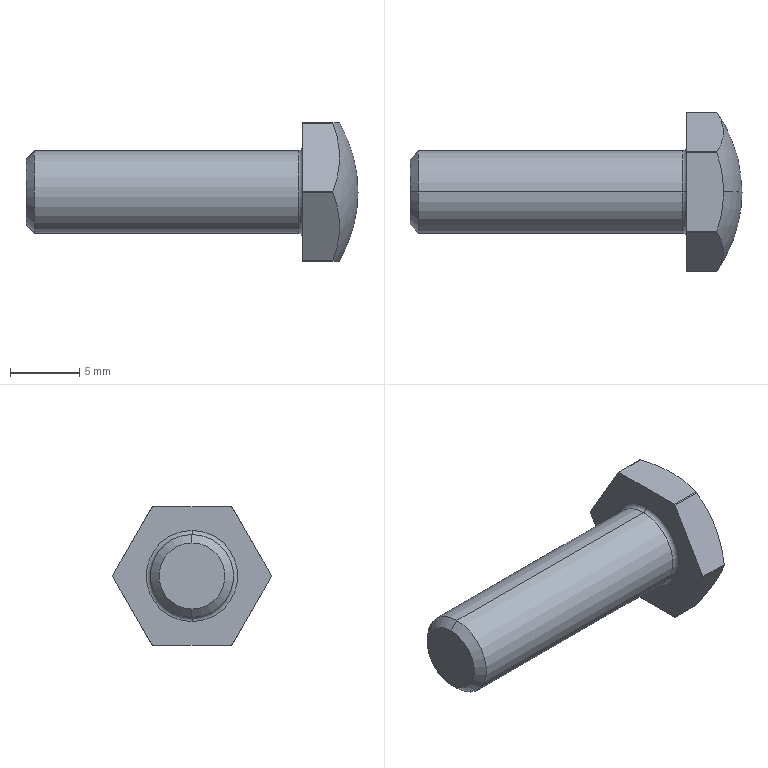Part | STEP file | SSTBB6-20-Part-1 | 1 solid | 22 faces | box 24 x 11.5 x 10 mm | volume 845.656 mm3 | cylinder 8 | plane 8 | cone 2 | torus 2 | sphere 2 | commonest cylinder face diameters 11.5 x6 6 x2
STEP:
#1=CARTESIAN_POINT('',(0.,0.,2.387));
#2=VERTEX_POINT('',#1);
#3=CARTESIAN_POINT('',(0.,0.,-2.387));
#4=VERTEX_POINT('',#3);
#5=CARTESIAN_POINT('',(0.,0.,0.));
#6=DIRECTION('',(-1.,0.,0.));
#7=DIRECTION('',(0.,0.,1.));
#8=AXIS2_PLACEMENT_3D('',#5,#6,#7);
#9=CIRCLE('',#8,2.387);
#10=EDGE_CURVE('',#2,#4,#9,.T.);
#11=ORIENTED_EDGE('',*,*,#10,.F.);
#12=CARTESIAN_POINT('',(0.6135,0.,3.));
#13=VERTEX_POINT('',#12);
#14=CARTESIAN_POINT('',(0.6135,0.,3.));
#15=DIRECTION('',(0.7071,0.,0.7071));
#16=VECTOR('',#15,1000.);
#17=LINE('',#14,#16);
#18=EDGE_CURVE('',#2,#13,#17,.T.);
#19=ORIENTED_EDGE('',*,*,#18,.T.);
#20=CARTESIAN_POINT('',(0.6135,0.,-3.));
#21=VERTEX_POINT('',#20);
#22=CARTESIAN_POINT('',(0.6135,0.,0.));
#23=DIRECTION('',(-1.,0.,0.));
#24=DIRECTION('',(0.,0.,1.));
#25=AXIS2_PLACEMENT_3D('',#22,#23,#24);
#26=CIRCLE('',#25,3.);
#27=EDGE_CURVE('',#13,#21,#26,.T.);
#28=ORIENTED_EDGE('',*,*,#27,.T.);
#29=CARTESIAN_POINT('',(0.6135,0.,-3.));
#30=DIRECTION('',(0.7071,0.,-0.7071));
#31=VECTOR('',#30,1000.);
#32=LINE('',#29,#31);
#33=EDGE_CURVE('',#4,#21,#32,.T.);
#34=ORIENTED_EDGE('',*,*,#33,.F.);
#35=EDGE_LOOP('',(#11,#19,#28,#34));
#36=FACE_OUTER_BOUND('',#35,.T.);
#37=CARTESIAN_POINT('',(0.6135,0.,0.));
#38=DIRECTION('',(1.,0.,0.));
#39=DIRECTION('',(0.,0.,-1.));
#40=AXIS2_PLACEMENT_3D('',#37,#38,#39);
#41=CONICAL_SURFACE('',#40,3.,0.7854);
#42=ADVANCED_FACE('',(#36),#41,.T.);
#43=CARTESIAN_POINT('',(19.7,0.,3.));
#44=VERTEX_POINT('',#43);
#45=CARTESIAN_POINT('',(19.7,0.,-3.));
#46=VERTEX_POINT('',#45);
#47=CARTESIAN_POINT('',(19.7,0.,0.));
#48=DIRECTION('',(-1.,0.,0.));
#49=DIRECTION('',(0.,0.,1.));
#50=AXIS2_PLACEMENT_3D('',#47,#48,#49);
#51=CIRCLE('',#50,3.);
#52=EDGE_CURVE('',#44,#46,#51,.T.);
#53=ORIENTED_EDGE('',*,*,#52,.T.);
#54=CARTESIAN_POINT('',(0.,0.,-3.));
#55=DIRECTION('',(-1.,0.,0.));
#56=VECTOR('',#55,1000.);
#57=LINE('',#54,#56);
#58=EDGE_CURVE('',#46,#21,#57,.T.);
#59=ORIENTED_EDGE('',*,*,#58,.T.);
#60=ORIENTED_EDGE('',*,*,#27,.F.);
#61=CARTESIAN_POINT('',(0.,0.,3.));
#62=DIRECTION('',(-1.,0.,0.));
#63=VECTOR('',#62,1000.);
#64=LINE('',#61,#63);
#65=EDGE_CURVE('',#44,#13,#64,.T.);
#66=ORIENTED_EDGE('',*,*,#65,.F.);
#67=EDGE_LOOP('',(#53,#59,#60,#66));
#68=FACE_OUTER_BOUND('',#67,.T.);
#69=CARTESIAN_POINT('',(0.,0.,0.));
#70=DIRECTION('',(-1.,0.,0.));
#71=DIRECTION('',(0.,0.,1.));
#72=AXIS2_PLACEMENT_3D('',#69,#70,#71);
#73=CYLINDRICAL_SURFACE('',#72,3.);
#74=ADVANCED_FACE('',(#68),#73,.T.);
#75=CARTESIAN_POINT('',(19.7,0.,0.));
#76=DIRECTION('',(-1.,0.,0.));
#77=DIRECTION('',(0.,0.,1.));
#78=AXIS2_PLACEMENT_3D('',#75,#76,#77);
#79=CIRCLE('',#78,3.);
#80=EDGE_CURVE('',#46,#44,#79,.T.);
#81=ORIENTED_EDGE('',*,*,#80,.F.);
#82=CARTESIAN_POINT('',(20.,0.,-3.3));
#83=VERTEX_POINT('',#82);
#84=CARTESIAN_POINT('',(19.7,0.,-3.3));
#85=DIRECTION('',(0.,1.,0.));
#86=DIRECTION('',(0.,0.,1.));
#87=AXIS2_PLACEMENT_3D('',#84,#85,#86);
#88=CIRCLE('',#87,0.3);
#89=EDGE_CURVE('',#46,#83,#88,.T.);
#90=ORIENTED_EDGE('',*,*,#89,.T.);
#91=CARTESIAN_POINT('',(20.,0.,3.3));
#92=VERTEX_POINT('',#91);
#93=CARTESIAN_POINT('',(20.,0.,0.));
#94=DIRECTION('',(-1.,0.,0.));
#95=DIRECTION('',(0.,0.,1.));
#96=AXIS2_PLACEMENT_3D('',#93,#94,#95);
#97=CIRCLE('',#96,3.3);
#98=EDGE_CURVE('',#83,#92,#97,.T.);
#99=ORIENTED_EDGE('',*,*,#98,.T.);
#100=CARTESIAN_POINT('',(19.7,0.,3.3));
#101=DIRECTION('',(0.,-1.,0.));
#102=DIRECTION('',(0.,0.,-1.));
#103=AXIS2_PLACEMENT_3D('',#100,#101,#102);
#104=CIRCLE('',#103,0.3);
#105=EDGE_CURVE('',#44,#92,#104,.T.);
#106=ORIENTED_EDGE('',*,*,#105,.F.);
#107=EDGE_LOOP('',(#81,#90,#99,#106));
#108=FACE_OUTER_BOUND('',#107,.T.);
#109=CARTESIAN_POINT('',(19.7,0.,0.));
#110=DIRECTION('',(-1.,0.,0.));
#111=DIRECTION('',(0.,0.,1.));
#112=AXIS2_PLACEMENT_3D('',#109,#110,#111);
#113=TOROIDAL_SURFACE('',#112,3.3,0.3);
#114=ADVANCED_FACE('',(#108),#113,.F.);
#115=CARTESIAN_POINT('',(24.,0.,0.));
#116=VERTEX_POINT('',#115);
#117=CARTESIAN_POINT('',(22.66,0.,5.));
#118=VERTEX_POINT('',#117);
#119=CARTESIAN_POINT('',(14.,0.,0.));
#120=DIRECTION('',(0.,-1.,0.));
#121=DIRECTION('',(0.,0.,-1.));
#122=AXIS2_PLACEMENT_3D('',#119,#120,#121);
#123=CIRCLE('',#122,10.);
#124=EDGE_CURVE('',#116,#118,#123,.T.);
#125=ORIENTED_EDGE('',*,*,#124,.F.);
#126=CARTESIAN_POINT('',(22.66,0.,-5.));
#127=VERTEX_POINT('',#126);
#128=CARTESIAN_POINT('',(14.,0.,0.));
#129=DIRECTION('',(0.,1.,0.));
#130=DIRECTION('',(0.,0.,1.));
#131=AXIS2_PLACEMENT_3D('',#128,#129,#130);
#132=CIRCLE('',#131,10.);
#133=EDGE_CURVE('',#116,#127,#132,.T.);
#134=ORIENTED_EDGE('',*,*,#133,.T.);
#135=CARTESIAN_POINT('',(22.182,2.839,-5.));
#136=VERTEX_POINT('',#135);
#137=CARTESIAN_POINT('',(14.,0.,-5.));
#138=DIRECTION('',(0.,0.,1.));
#139=DIRECTION('',(-1.,0.,0.));
#140=AXIS2_PLACEMENT_3D('',#137,#138,#139);
#141=CIRCLE('',#140,8.66);
#142=EDGE_CURVE('',#127,#136,#141,.T.);
#143=ORIENTED_EDGE('',*,*,#142,.T.);
#144=CARTESIAN_POINT('',(22.182,2.91,-4.959));
#145=VERTEX_POINT('',#144);
#146=CARTESIAN_POINT('',(22.182,0.,0.));
#147=DIRECTION('',(-1.,0.,0.));
#148=DIRECTION('',(0.,0.,1.));
#149=AXIS2_PLACEMENT_3D('',#146,#147,#148);
#150=CIRCLE('',#149,5.75);
#151=EDGE_CURVE('',#145,#136,#150,.T.);
#152=ORIENTED_EDGE('',*,*,#151,.F.);
#153=CARTESIAN_POINT('',(22.182,5.75,-0.04096));
#154=VERTEX_POINT('',#153);
#155=CARTESIAN_POINT('',(14.,4.33,-2.5));
#156=DIRECTION('',(0.,-0.866,0.5));
#157=DIRECTION('',(0.,-0.5,-0.866));
#158=AXIS2_PLACEMENT_3D('',#155,#156,#157);
#159=CIRCLE('',#158,8.66);
#160=EDGE_CURVE('',#145,#154,#159,.T.);
#161=ORIENTED_EDGE('',*,*,#160,.T.);
#162=CARTESIAN_POINT('',(22.182,5.75,0.04096));
#163=VERTEX_POINT('',#162);
#164=CARTESIAN_POINT('',(22.182,0.,0.));
#165=DIRECTION('',(-1.,0.,0.));
#166=DIRECTION('',(0.,0.,1.));
#167=AXIS2_PLACEMENT_3D('',#164,#165,#166);
#168=CIRCLE('',#167,5.75);
#169=EDGE_CURVE('',#163,#154,#168,.T.);
#170=ORIENTED_EDGE('',*,*,#169,.F.);
#171=CARTESIAN_POINT('',(22.182,2.91,4.959));
#172=VERTEX_POINT('',#171);
#173=CARTESIAN_POINT('',(14.,4.33,2.5));
#174=DIRECTION('',(0.,-0.866,-0.5));
#175=DIRECTION('',(0.,0.5,-0.866));
#176=AXIS2_PLACEMENT_3D('',#173,#174,#175);
#177=CIRCLE('',#176,8.66);
#178=EDGE_CURVE('',#163,#172,#177,.T.);
#179=ORIENTED_EDGE('',*,*,#178,.T.);
#180=CARTESIAN_POINT('',(22.182,2.839,5.));
#181=VERTEX_POINT('',#180);
#182=CARTESIAN_POINT('',(22.182,0.,0.));
#183=DIRECTION('',(-1.,0.,0.));
#184=DIRECTION('',(0.,0.,1.));
#185=AXIS2_PLACEMENT_3D('',#182,#183,#184);
#186=CIRCLE('',#185,5.75);
#187=EDGE_CURVE('',#181,#172,#186,.T.);
#188=ORIENTED_EDGE('',*,*,#187,.F.);
#189=CARTESIAN_POINT('',(14.,0.,5.));
#190=DIRECTION('',(0.,0.,-1.));
#191=DIRECTION('',(1.,0.,0.));
#192=AXIS2_PLACEMENT_3D('',#189,#190,#191);
#193=CIRCLE('',#192,8.66);
#194=EDGE_CURVE('',#181,#118,#193,.T.);
#195=ORIENTED_EDGE('',*,*,#194,.T.);
#196=EDGE_LOOP('',(#125,#134,#143,#152,#161,#170,#179,#188,#195));
#197=FACE_OUTER_BOUND('',#196,.T.);
#198=CARTESIAN_POINT('',(14.,0.,0.));
#199=DIRECTION('',(0.,1.,0.));
#200=DIRECTION('',(0.,0.,1.));
#201=AXIS2_PLACEMENT_3D('',#198,#199,#200);
#202=SPHERICAL_SURFACE('',#201,10.);
#203=ADVANCED_FACE('',(#197),#202,.T.);
#204=ORIENTED_EDGE('',*,*,#133,.F.);
#205=ORIENTED_EDGE('',*,*,#124,.T.);
#206=CARTESIAN_POINT('',(22.182,-2.839,5.));
#207=VERTEX_POINT('',#206);
#208=CARTESIAN_POINT('',(14.,0.,5.));
#209=DIRECTION('',(0.,0.,-1.));
#210=DIRECTION('',(1.,0.,0.));
#211=AXIS2_PLACEMENT_3D('',#208,#209,#210);
#212=CIRCLE('',#211,8.66);
#213=EDGE_CURVE('',#118,#207,#212,.T.);
#214=ORIENTED_EDGE('',*,*,#213,.T.);
#215=CARTESIAN_POINT('',(22.182,-2.91,4.959));
#216=VERTEX_POINT('',#215);
#217=CARTESIAN_POINT('',(22.182,0.,0.));
#218=DIRECTION('',(-1.,0.,0.));
#219=DIRECTION('',(0.,0.,1.));
#220=AXIS2_PLACEMENT_3D('',#217,#218,#219);
#221=CIRCLE('',#220,5.75);
#222=EDGE_CURVE('',#216,#207,#221,.T.);
#223=ORIENTED_EDGE('',*,*,#222,.F.);
#224=CARTESIAN_POINT('',(22.182,-5.75,0.04096));
#225=VERTEX_POINT('',#224);
#226=CARTESIAN_POINT('',(14.,-4.33,2.5));
#227=DIRECTION('',(0.,0.866,-0.5));
#228=DIRECTION('',(0.,0.5,0.866));
#229=AXIS2_PLACEMENT_3D('',#226,#227,#228);
#230=CIRCLE('',#229,8.66);
#231=EDGE_CURVE('',#216,#225,#230,.T.);
#232=ORIENTED_EDGE('',*,*,#231,.T.);
#233=CARTESIAN_POINT('',(22.182,-5.75,-0.04096));
#234=VERTEX_POINT('',#233);
#235=CARTESIAN_POINT('',(22.182,0.,0.));
#236=DIRECTION('',(-1.,0.,0.));
#237=DIRECTION('',(0.,0.,1.));
#238=AXIS2_PLACEMENT_3D('',#235,#236,#237);
#239=CIRCLE('',#238,5.75);
#240=EDGE_CURVE('',#234,#225,#239,.T.);
#241=ORIENTED_EDGE('',*,*,#240,.F.);
#242=CARTESIAN_POINT('',(22.182,-2.91,-4.959));
#243=VERTEX_POINT('',#242);
#244=CARTESIAN_POINT('',(14.,-4.33,-2.5));
#245=DIRECTION('',(0.,0.866,0.5));
#246=DIRECTION('',(0.,-0.5,0.866));
#247=AXIS2_PLACEMENT_3D('',#244,#245,#246);
#248=CIRCLE('',#247,8.66);
#249=EDGE_CURVE('',#234,#243,#248,.T.);
#250=ORIENTED_EDGE('',*,*,#249,.T.);
#251=CARTESIAN_POINT('',(22.182,-2.839,-5.));
#252=VERTEX_POINT('',#251);
#253=CARTESIAN_POINT('',(22.182,0.,0.));
#254=DIRECTION('',(-1.,0.,0.));
#255=DIRECTION('',(0.,0.,1.));
#256=AXIS2_PLACEMENT_3D('',#253,#254,#255);
#257=CIRCLE('',#256,5.75);
#258=EDGE_CURVE('',#252,#243,#257,.T.);
#259=ORIENTED_EDGE('',*,*,#258,.F.);
#260=CARTESIAN_POINT('',(14.,0.,-5.));
#261=DIRECTION('',(0.,0.,1.));
#262=DIRECTION('',(-1.,0.,0.));
#263=AXIS2_PLACEMENT_3D('',#260,#261,#262);
#264=CIRCLE('',#263,8.66);
#265=EDGE_CURVE('',#252,#127,#264,.T.);
#266=ORIENTED_EDGE('',*,*,#265,.T.);
#267=EDGE_LOOP('',(#204,#205,#214,#223,#232,#241,#250,#259,#266));
#268=FACE_OUTER_BOUND('',#267,.T.);
#269=CARTESIAN_POINT('',(14.,0.,0.));
#270=DIRECTION('',(0.,1.,0.));
#271=DIRECTION('',(0.,0.,1.));
#272=AXIS2_PLACEMENT_3D('',#269,#270,#271);
#273=SPHERICAL_SURFACE('',#272,10.);
#274=ADVANCED_FACE('',(#268),#273,.T.);
#275=CARTESIAN_POINT('',(20.,-2.839,-5.));
#276=VERTEX_POINT('',#275);
#277=CARTESIAN_POINT('',(0.,-2.839,-5.));
#278=DIRECTION('',(-1.,0.,0.));
#279=VECTOR('',#278,1000.);
#280=LINE('',#277,#279);
#281=EDGE_CURVE('',#252,#276,#280,.T.);
#282=ORIENTED_EDGE('',*,*,#281,.F.);
#283=ORIENTED_EDGE('',*,*,#258,.T.);
#284=CARTESIAN_POINT('',(20.,-2.91,-4.959));
#285=VERTEX_POINT('',#284);
#286=CARTESIAN_POINT('',(0.,-2.91,-4.959));
#287=DIRECTION('',(1.,0.,0.));
#288=VECTOR('',#287,1000.);
#289=LINE('',#286,#288);
#290=EDGE_CURVE('',#285,#243,#289,.T.);
#291=ORIENTED_EDGE('',*,*,#290,.F.);
#292=CARTESIAN_POINT('',(20.,0.,0.));
#293=DIRECTION('',(-1.,0.,0.));
#294=DIRECTION('',(0.,0.,1.));
#295=AXIS2_PLACEMENT_3D('',#292,#293,#294);
#296=CIRCLE('',#295,5.75);
#297=EDGE_CURVE('',#276,#285,#296,.T.);
#298=ORIENTED_EDGE('',*,*,#297,.F.);
#299=EDGE_LOOP('',(#282,#283,#291,#298));
#300=FACE_OUTER_BOUND('',#299,.T.);
#301=CARTESIAN_POINT('',(0.,0.,0.));
#302=DIRECTION('',(-1.,0.,0.));
#303=DIRECTION('',(0.,0.,1.));
#304=AXIS2_PLACEMENT_3D('',#301,#302,#303);
#305=CYLINDRICAL_SURFACE('',#304,5.75);
#306=ADVANCED_FACE('',(#300),#305,.T.);
#307=CARTESIAN_POINT('',(20.,2.839,-5.));
#308=VERTEX_POINT('',#307);
#309=CARTESIAN_POINT('',(0.,2.839,-5.));
#310=DIRECTION('',(1.,0.,0.));
#311=VECTOR('',#310,1000.);
#312=LINE('',#309,#311);
#313=EDGE_CURVE('',#308,#136,#312,.T.);
#314=ORIENTED_EDGE('',*,*,#313,.F.);
#315=CARTESIAN_POINT('',(20.,2.91,-4.959));
#316=VERTEX_POINT('',#315);
#317=CARTESIAN_POINT('',(20.,0.,0.));
#318=DIRECTION('',(-1.,0.,0.));
#319=DIRECTION('',(0.,0.,1.));
#320=AXIS2_PLACEMENT_3D('',#317,#318,#319);
#321=CIRCLE('',#320,5.75);
#322=EDGE_CURVE('',#316,#308,#321,.T.);
#323=ORIENTED_EDGE('',*,*,#322,.F.);
#324=CARTESIAN_POINT('',(0.,2.91,-4.959));
#325=DIRECTION('',(-1.,0.,0.));
#326=VECTOR('',#325,1000.);
#327=LINE('',#324,#326);
#328=EDGE_CURVE('',#145,#316,#327,.T.);
#329=ORIENTED_EDGE('',*,*,#328,.F.);
#330=ORIENTED_EDGE('',*,*,#151,.T.);
#331=EDGE_LOOP('',(#314,#323,#329,#330));
#332=FACE_OUTER_BOUND('',#331,.T.);
#333=CARTESIAN_POINT('',(0.,0.,0.));
#334=DIRECTION('',(-1.,0.,0.));
#335=DIRECTION('',(0.,0.,1.));
#336=AXIS2_PLACEMENT_3D('',#333,#334,#335);
#337=CYLINDRICAL_SURFACE('',#336,5.75);
#338=ADVANCED_FACE('',(#332),#337,.T.);
#339=CARTESIAN_POINT('',(20.,5.75,-0.04096));
#340=VERTEX_POINT('',#339);
#341=CARTESIAN_POINT('',(0.,5.75,-0.04096));
#342=DIRECTION('',(1.,0.,0.));
#343=VECTOR('',#342,1000.);
#344=LINE('',#341,#343);
#345=EDGE_CURVE('',#340,#154,#344,.T.);
#346=ORIENTED_EDGE('',*,*,#345,.F.);
#347=CARTESIAN_POINT('',(20.,5.75,0.04096));
#348=VERTEX_POINT('',#347);
#349=CARTESIAN_POINT('',(20.,0.,0.));
#350=DIRECTION('',(-1.,0.,0.));
#351=DIRECTION('',(0.,0.,1.));
#352=AXIS2_PLACEMENT_3D('',#349,#350,#351);
#353=CIRCLE('',#352,5.75);
#354=EDGE_CURVE('',#348,#340,#353,.T.);
#355=ORIENTED_EDGE('',*,*,#354,.F.);
#356=CARTESIAN_POINT('',(0.,5.75,0.04096));
#357=DIRECTION('',(-1.,0.,0.));
#358=VECTOR('',#357,1000.);
#359=LINE('',#356,#358);
#360=EDGE_CURVE('',#163,#348,#359,.T.);
#361=ORIENTED_EDGE('',*,*,#360,.F.);
#362=ORIENTED_EDGE('',*,*,#169,.T.);
#363=EDGE_LOOP('',(#346,#355,#361,#362));
#364=FACE_OUTER_BOUND('',#363,.T.);
#365=CARTESIAN_POINT('',(0.,0.,0.));
#366=DIRECTION('',(-1.,0.,0.));
#367=DIRECTION('',(0.,0.,1.));
#368=AXIS2_PLACEMENT_3D('',#365,#366,#367);
#369=CYLINDRICAL_SURFACE('',#368,5.75);
#370=ADVANCED_FACE('',(#364),#369,.T.);
#371=CARTESIAN_POINT('',(20.,2.91,4.959));
#372=VERTEX_POINT('',#371);
#373=CARTESIAN_POINT('',(0.,2.91,4.959));
#374=DIRECTION('',(1.,0.,0.));
#375=VECTOR('',#374,1000.);
#376=LINE('',#373,#375);
#377=EDGE_CURVE('',#372,#172,#376,.T.);
#378=ORIENTED_EDGE('',*,*,#377,.F.);
#379=CARTESIAN_POINT('',(20.,2.839,5.));
#380=VERTEX_POINT('',#379);
#381=CARTESIAN_POINT('',(20.,0.,0.));
#382=DIRECTION('',(-1.,0.,0.));
#383=DIRECTION('',(0.,0.,1.));
#384=AXIS2_PLACEMENT_3D('',#381,#382,#383);
#385=CIRCLE('',#384,5.75);
#386=EDGE_CURVE('',#380,#372,#385,.T.);
#387=ORIENTED_EDGE('',*,*,#386,.F.);
#388=CARTESIAN_POINT('',(0.,2.839,5.));
#389=DIRECTION('',(-1.,0.,0.));
#390=VECTOR('',#389,1000.);
#391=LINE('',#388,#390);
#392=EDGE_CURVE('',#181,#380,#391,.T.);
#393=ORIENTED_EDGE('',*,*,#392,.F.);
#394=ORIENTED_EDGE('',*,*,#187,.T.);
#395=EDGE_LOOP('',(#378,#387,#393,#394));
#396=FACE_OUTER_BOUND('',#395,.T.);
#397=CARTESIAN_POINT('',(0.,0.,0.));
#398=DIRECTION('',(-1.,0.,0.));
#399=DIRECTION('',(0.,0.,1.));
#400=AXIS2_PLACEMENT_3D('',#397,#398,#399);
#401=CYLINDRICAL_SURFACE('',#400,5.75);
#402=ADVANCED_FACE('',(#396),#401,.T.);
#403=CARTESIAN_POINT('',(20.,-2.839,5.));
#404=VERTEX_POINT('',#403);
#405=CARTESIAN_POINT('',(0.,-2.839,5.));
#406=DIRECTION('',(1.,0.,0.));
#407=VECTOR('',#406,1000.);
#408=LINE('',#405,#407);
#409=EDGE_CURVE('',#404,#207,#408,.T.);
#410=ORIENTED_EDGE('',*,*,#409,.F.);
#411=CARTESIAN_POINT('',(20.,-2.91,4.959));
#412=VERTEX_POINT('',#411);
#413=CARTESIAN_POINT('',(20.,0.,0.));
#414=DIRECTION('',(-1.,0.,0.));
#415=DIRECTION('',(0.,0.,1.));
#416=AXIS2_PLACEMENT_3D('',#413,#414,#415);
#417=CIRCLE('',#416,5.75);
#418=EDGE_CURVE('',#412,#404,#417,.T.);
#419=ORIENTED_EDGE('',*,*,#418,.F.);
#420=CARTESIAN_POINT('',(0.,-2.91,4.959));
#421=DIRECTION('',(-1.,0.,0.));
#422=VECTOR('',#421,1000.);
#423=LINE('',#420,#422);
#424=EDGE_CURVE('',#216,#412,#423,.T.);
#425=ORIENTED_EDGE('',*,*,#424,.F.);
#426=ORIENTED_EDGE('',*,*,#222,.T.);
#427=EDGE_LOOP('',(#410,#419,#425,#426));
#428=FACE_OUTER_BOUND('',#427,.T.);
#429=CARTESIAN_POINT('',(0.,0.,0.));
#430=DIRECTION('',(-1.,0.,0.));
#431=DIRECTION('',(0.,0.,1.));
#432=AXIS2_PLACEMENT_3D('',#429,#430,#431);
#433=CYLINDRICAL_SURFACE('',#432,5.75);
#434=ADVANCED_FACE('',(#428),#433,.T.);
#435=CARTESIAN_POINT('',(20.,-5.75,0.04096));
#436=VERTEX_POINT('',#435);
#437=CARTESIAN_POINT('',(0.,-5.75,0.04096));
#438=DIRECTION('',(1.,0.,0.));
#439=VECTOR('',#438,1000.);
#440=LINE('',#437,#439);
#441=EDGE_CURVE('',#436,#225,#440,.T.);
#442=ORIENTED_EDGE('',*,*,#441,.F.);
#443=CARTESIAN_POINT('',(20.,-5.75,-0.04096));
#444=VERTEX_POINT('',#443);
#445=CARTESIAN_POINT('',(20.,0.,0.));
#446=DIRECTION('',(-1.,0.,0.));
#447=DIRECTION('',(0.,0.,1.));
#448=AXIS2_PLACEMENT_3D('',#445,#446,#447);
#449=CIRCLE('',#448,5.75);
#450=EDGE_CURVE('',#444,#436,#449,.T.);
#451=ORIENTED_EDGE('',*,*,#450,.F.);
#452=CARTESIAN_POINT('',(0.,-5.75,-0.04096));
#453=DIRECTION('',(-1.,0.,0.));
#454=VECTOR('',#453,1000.);
#455=LINE('',#452,#454);
#456=EDGE_CURVE('',#234,#444,#455,.T.);
#457=ORIENTED_EDGE('',*,*,#456,.F.);
#458=ORIENTED_EDGE('',*,*,#240,.T.);
#459=EDGE_LOOP('',(#442,#451,#457,#458));
#460=FACE_OUTER_BOUND('',#459,.T.);
#461=CARTESIAN_POINT('',(0.,0.,0.));
#462=DIRECTION('',(-1.,0.,0.));
#463=DIRECTION('',(0.,0.,1.));
#464=AXIS2_PLACEMENT_3D('',#461,#462,#463);
#465=CYLINDRICAL_SURFACE('',#464,5.75);
#466=ADVANCED_FACE('',(#460),#465,.T.);
#467=CARTESIAN_POINT('',(20.,0.,0.));
#468=DIRECTION('',(-1.,0.,0.));
#469=DIRECTION('',(0.,0.,1.));
#470=AXIS2_PLACEMENT_3D('',#467,#468,#469);
#471=CIRCLE('',#470,3.3);
#472=EDGE_CURVE('',#92,#83,#471,.T.);
#473=ORIENTED_EDGE('',*,*,#472,.F.);
#474=ORIENTED_EDGE('',*,*,#98,.F.);
#475=EDGE_LOOP('',(#473,#474));
#476=FACE_BOUND('',#475,.T.);
#477=CARTESIAN_POINT('',(20.,0.,-5.));
#478=DIRECTION('',(0.,1.,0.));
#479=VECTOR('',#478,1000.);
#480=LINE('',#477,#479);
#481=EDGE_CURVE('',#276,#308,#480,.T.);
#482=ORIENTED_EDGE('',*,*,#481,.F.);
#483=ORIENTED_EDGE('',*,*,#297,.T.);
#484=CARTESIAN_POINT('',(20.,-6.82,1.812));
#485=DIRECTION('',(0.,0.5,-0.866));
#486=VECTOR('',#485,1000.);
#487=LINE('',#484,#486);
#488=EDGE_CURVE('',#444,#285,#487,.T.);
#489=ORIENTED_EDGE('',*,*,#488,.F.);
#490=ORIENTED_EDGE('',*,*,#450,.T.);
#491=CARTESIAN_POINT('',(20.,-1.84,6.812));
#492=DIRECTION('',(0.,-0.5,-0.866));
#493=VECTOR('',#492,1000.);
#494=LINE('',#491,#493);
#495=EDGE_CURVE('',#412,#436,#494,.T.);
#496=ORIENTED_EDGE('',*,*,#495,.F.);
#497=ORIENTED_EDGE('',*,*,#418,.T.);
#498=CARTESIAN_POINT('',(20.,0.,5.));
#499=DIRECTION('',(0.,-1.,0.));
#500=VECTOR('',#499,1000.);
#501=LINE('',#498,#500);
#502=EDGE_CURVE('',#380,#404,#501,.T.);
#503=ORIENTED_EDGE('',*,*,#502,.F.);
#504=ORIENTED_EDGE('',*,*,#386,.T.);
#505=CARTESIAN_POINT('',(20.,1.84,6.812));
#506=DIRECTION('',(0.,-0.5,0.866));
#507=VECTOR('',#506,1000.);
#508=LINE('',#505,#507);
#509=EDGE_CURVE('',#348,#372,#508,.T.);
#510=ORIENTED_EDGE('',*,*,#509,.F.);
#511=ORIENTED_EDGE('',*,*,#354,.T.);
#512=CARTESIAN_POINT('',(20.,6.82,1.812));
#513=DIRECTION('',(0.,0.5,0.866));
#514=VECTOR('',#513,1000.);
#515=LINE('',#512,#514);
#516=EDGE_CURVE('',#316,#340,#515,.T.);
#517=ORIENTED_EDGE('',*,*,#516,.F.);
#518=ORIENTED_EDGE('',*,*,#322,.T.);
#519=EDGE_LOOP('',(#482,#483,#489,#490,#496,#497,#503,#504,#510,#511,#517,#518));
#520=FACE_OUTER_BOUND('',#519,.T.);
#521=CARTESIAN_POINT('',(20.,0.,5.75));
#522=DIRECTION('',(1.,0.,0.));
#523=DIRECTION('',(0.,0.,-1.));
#524=AXIS2_PLACEMENT_3D('',#521,#522,#523);
#525=PLANE('',#524);
#526=ADVANCED_FACE('',(#476,#520),#525,.F.);
#527=ORIENTED_EDGE('',*,*,#89,.F.);
#528=ORIENTED_EDGE('',*,*,#52,.F.);
#529=ORIENTED_EDGE('',*,*,#105,.T.);
#530=ORIENTED_EDGE('',*,*,#472,.T.);
#531=EDGE_LOOP('',(#527,#528,#529,#530));
#532=FACE_OUTER_BOUND('',#531,.T.);
#533=CARTESIAN_POINT('',(19.7,0.,0.));
#534=DIRECTION('',(-1.,0.,0.));
#535=DIRECTION('',(0.,0.,1.));
#536=AXIS2_PLACEMENT_3D('',#533,#534,#535);
#537=TOROIDAL_SURFACE('',#536,3.3,0.3);
#538=ADVANCED_FACE('',(#532),#537,.F.);
#539=ORIENTED_EDGE('',*,*,#58,.F.);
#540=ORIENTED_EDGE('',*,*,#80,.T.);
#541=ORIENTED_EDGE('',*,*,#65,.T.);
#542=CARTESIAN_POINT('',(0.6135,0.,0.));
#543=DIRECTION('',(-1.,0.,0.));
#544=DIRECTION('',(0.,0.,1.));
#545=AXIS2_PLACEMENT_3D('',#542,#543,#544);
#546=CIRCLE('',#545,3.);
#547=EDGE_CURVE('',#21,#13,#546,.T.);
#548=ORIENTED_EDGE('',*,*,#547,.F.);
#549=EDGE_LOOP('',(#539,#540,#541,#548));
#550=FACE_OUTER_BOUND('',#549,.T.);
#551=CARTESIAN_POINT('',(0.,0.,0.));
#552=DIRECTION('',(-1.,0.,0.));
#553=DIRECTION('',(0.,0.,1.));
#554=AXIS2_PLACEMENT_3D('',#551,#552,#553);
#555=CYLINDRICAL_SURFACE('',#554,3.);
#556=ADVANCED_FACE('',(#550),#555,.T.);
#557=ORIENTED_EDGE('',*,*,#18,.F.);
#558=CARTESIAN_POINT('',(0.,0.,0.));
#559=DIRECTION('',(-1.,0.,0.));
#560=DIRECTION('',(0.,0.,1.));
#561=AXIS2_PLACEMENT_3D('',#558,#559,#560);
#562=CIRCLE('',#561,2.387);
#563=EDGE_CURVE('',#4,#2,#562,.T.);
#564=ORIENTED_EDGE('',*,*,#563,.F.);
#565=ORIENTED_EDGE('',*,*,#33,.T.);
#566=ORIENTED_EDGE('',*,*,#547,.T.);
#567=EDGE_LOOP('',(#557,#564,#565,#566));
#568=FACE_OUTER_BOUND('',#567,.T.);
#569=CARTESIAN_POINT('',(0.6135,0.,0.));
#570=DIRECTION('',(1.,0.,0.));
#571=DIRECTION('',(0.,0.,-1.));
#572=AXIS2_PLACEMENT_3D('',#569,#570,#571);
#573=CONICAL_SURFACE('',#572,3.,0.7854);
#574=ADVANCED_FACE('',(#568),#573,.T.);
#575=ORIENTED_EDGE('',*,*,#563,.T.);
#576=ORIENTED_EDGE('',*,*,#10,.T.);
#577=EDGE_LOOP('',(#575,#576));
#578=FACE_OUTER_BOUND('',#577,.T.);
#579=CARTESIAN_POINT('',(0.,0.,2.387));
#580=DIRECTION('',(1.,0.,0.));
#581=DIRECTION('',(0.,0.,-1.));
#582=AXIS2_PLACEMENT_3D('',#579,#580,#581);
#583=PLANE('',#582);
#584=ADVANCED_FACE('',(#578),#583,.F.);
#585=ORIENTED_EDGE('',*,*,#456,.T.);
#586=ORIENTED_EDGE('',*,*,#488,.T.);
#587=ORIENTED_EDGE('',*,*,#290,.T.);
#588=ORIENTED_EDGE('',*,*,#249,.F.);
#589=EDGE_LOOP('',(#585,#586,#587,#588));
#590=FACE_OUTER_BOUND('',#589,.T.);
#591=CARTESIAN_POINT('',(24.,-2.887,-5.));
#592=DIRECTION('',(0.,-0.866,-0.5));
#593=DIRECTION('',(0.,-0.5,0.866));
#594=AXIS2_PLACEMENT_3D('',#591,#592,#593);
#595=PLANE('',#594);
#596=ADVANCED_FACE('',(#590),#595,.T.);
#597=ORIENTED_EDGE('',*,*,#424,.T.);
#598=ORIENTED_EDGE('',*,*,#495,.T.);
#599=ORIENTED_EDGE('',*,*,#441,.T.);
#600=ORIENTED_EDGE('',*,*,#231,.F.);
#601=EDGE_LOOP('',(#597,#598,#599,#600));
#602=FACE_OUTER_BOUND('',#601,.T.);
#603=CARTESIAN_POINT('',(24.,-5.774,0.));
#604=DIRECTION('',(0.,-0.866,0.5));
#605=DIRECTION('',(0.,0.5,0.866));
#606=AXIS2_PLACEMENT_3D('',#603,#604,#605);
#607=PLANE('',#606);
#608=ADVANCED_FACE('',(#602),#607,.T.);
#609=ORIENTED_EDGE('',*,*,#392,.T.);
#610=ORIENTED_EDGE('',*,*,#502,.T.);
#611=ORIENTED_EDGE('',*,*,#409,.T.);
#612=ORIENTED_EDGE('',*,*,#213,.F.);
#613=ORIENTED_EDGE('',*,*,#194,.F.);
#614=EDGE_LOOP('',(#609,#610,#611,#612,#613));
#615=FACE_OUTER_BOUND('',#614,.T.);
#616=CARTESIAN_POINT('',(24.,-2.887,5.));
#617=DIRECTION('',(0.,0.,1.));
#618=DIRECTION('',(1.,0.,0.));
#619=AXIS2_PLACEMENT_3D('',#616,#617,#618);
#620=PLANE('',#619);
#621=ADVANCED_FACE('',(#615),#620,.T.);
#622=ORIENTED_EDGE('',*,*,#360,.T.);
#623=ORIENTED_EDGE('',*,*,#509,.T.);
#624=ORIENTED_EDGE('',*,*,#377,.T.);
#625=ORIENTED_EDGE('',*,*,#178,.F.);
#626=EDGE_LOOP('',(#622,#623,#624,#625));
#627=FACE_OUTER_BOUND('',#626,.T.);
#628=CARTESIAN_POINT('',(24.,2.887,5.));
#629=DIRECTION('',(0.,0.866,0.5));
#630=DIRECTION('',(0.,0.5,-0.866));
#631=AXIS2_PLACEMENT_3D('',#628,#629,#630);
#632=PLANE('',#631);
#633=ADVANCED_FACE('',(#627),#632,.T.);
#634=ORIENTED_EDGE('',*,*,#328,.T.);
#635=ORIENTED_EDGE('',*,*,#516,.T.);
#636=ORIENTED_EDGE('',*,*,#345,.T.);
#637=ORIENTED_EDGE('',*,*,#160,.F.);
#638=EDGE_LOOP('',(#634,#635,#636,#637));
#639=FACE_OUTER_BOUND('',#638,.T.);
#640=CARTESIAN_POINT('',(24.,5.774,0.));
#641=DIRECTION('',(0.,0.866,-0.5));
#642=DIRECTION('',(0.,-0.5,-0.866));
#643=AXIS2_PLACEMENT_3D('',#640,#641,#642);
#644=PLANE('',#643);
#645=ADVANCED_FACE('',(#639),#644,.T.);
#646=ORIENTED_EDGE('',*,*,#281,.T.);
#647=ORIENTED_EDGE('',*,*,#481,.T.);
#648=ORIENTED_EDGE('',*,*,#313,.T.);
#649=ORIENTED_EDGE('',*,*,#142,.F.);
#650=ORIENTED_EDGE('',*,*,#265,.F.);
#651=EDGE_LOOP('',(#646,#647,#648,#649,#650));
#652=FACE_OUTER_BOUND('',#651,.T.);
#653=CARTESIAN_POINT('',(24.,2.887,-5.));
#654=DIRECTION('',(0.,0.,-1.));
#655=DIRECTION('',(-1.,0.,0.));
#656=AXIS2_PLACEMENT_3D('',#653,#654,#655);
#657=PLANE('',#656);
#658=ADVANCED_FACE('',(#652),#657,.T.);
#659=CLOSED_SHELL('',(#42,#74,#114,#203,#274,#306,#338,#370,#402,#434,#466,#526,#538,#556,#574,#584,#596,#608,#621,#633,#645,#658));
#660=MANIFOLD_SOLID_BREP('',#659);
#661=CARTESIAN_POINT('',(0.,0.,0.));
#662=DIRECTION('',(0.,0.,1.));
#663=DIRECTION('',(1.,0.,0.));
#664=AXIS2_PLACEMENT_3D('',#661,#662,#663);
#665=(LENGTH_UNIT()NAMED_UNIT(*)SI_UNIT(.MILLI.,.METRE.));
#666=UNCERTAINTY_MEASURE_WITH_UNIT(LENGTH_MEASURE(0.00001),#665,'','');
#667=(NAMED_UNIT(*)PLANE_ANGLE_UNIT()SI_UNIT($,.RADIAN.));
#668=(NAMED_UNIT(*)SI_UNIT($,.STERADIAN.)SOLID_ANGLE_UNIT());
#669=(GEOMETRIC_REPRESENTATION_CONTEXT(3)GLOBAL_UNCERTAINTY_ASSIGNED_CONTEXT((#666))GLOBAL_UNIT_ASSIGNED_CONTEXT((#665,#667,#668))REPRESENTATION_CONTEXT('',''));
#670=ADVANCED_BREP_SHAPE_REPRESENTATION('',(#660,#664),#669);